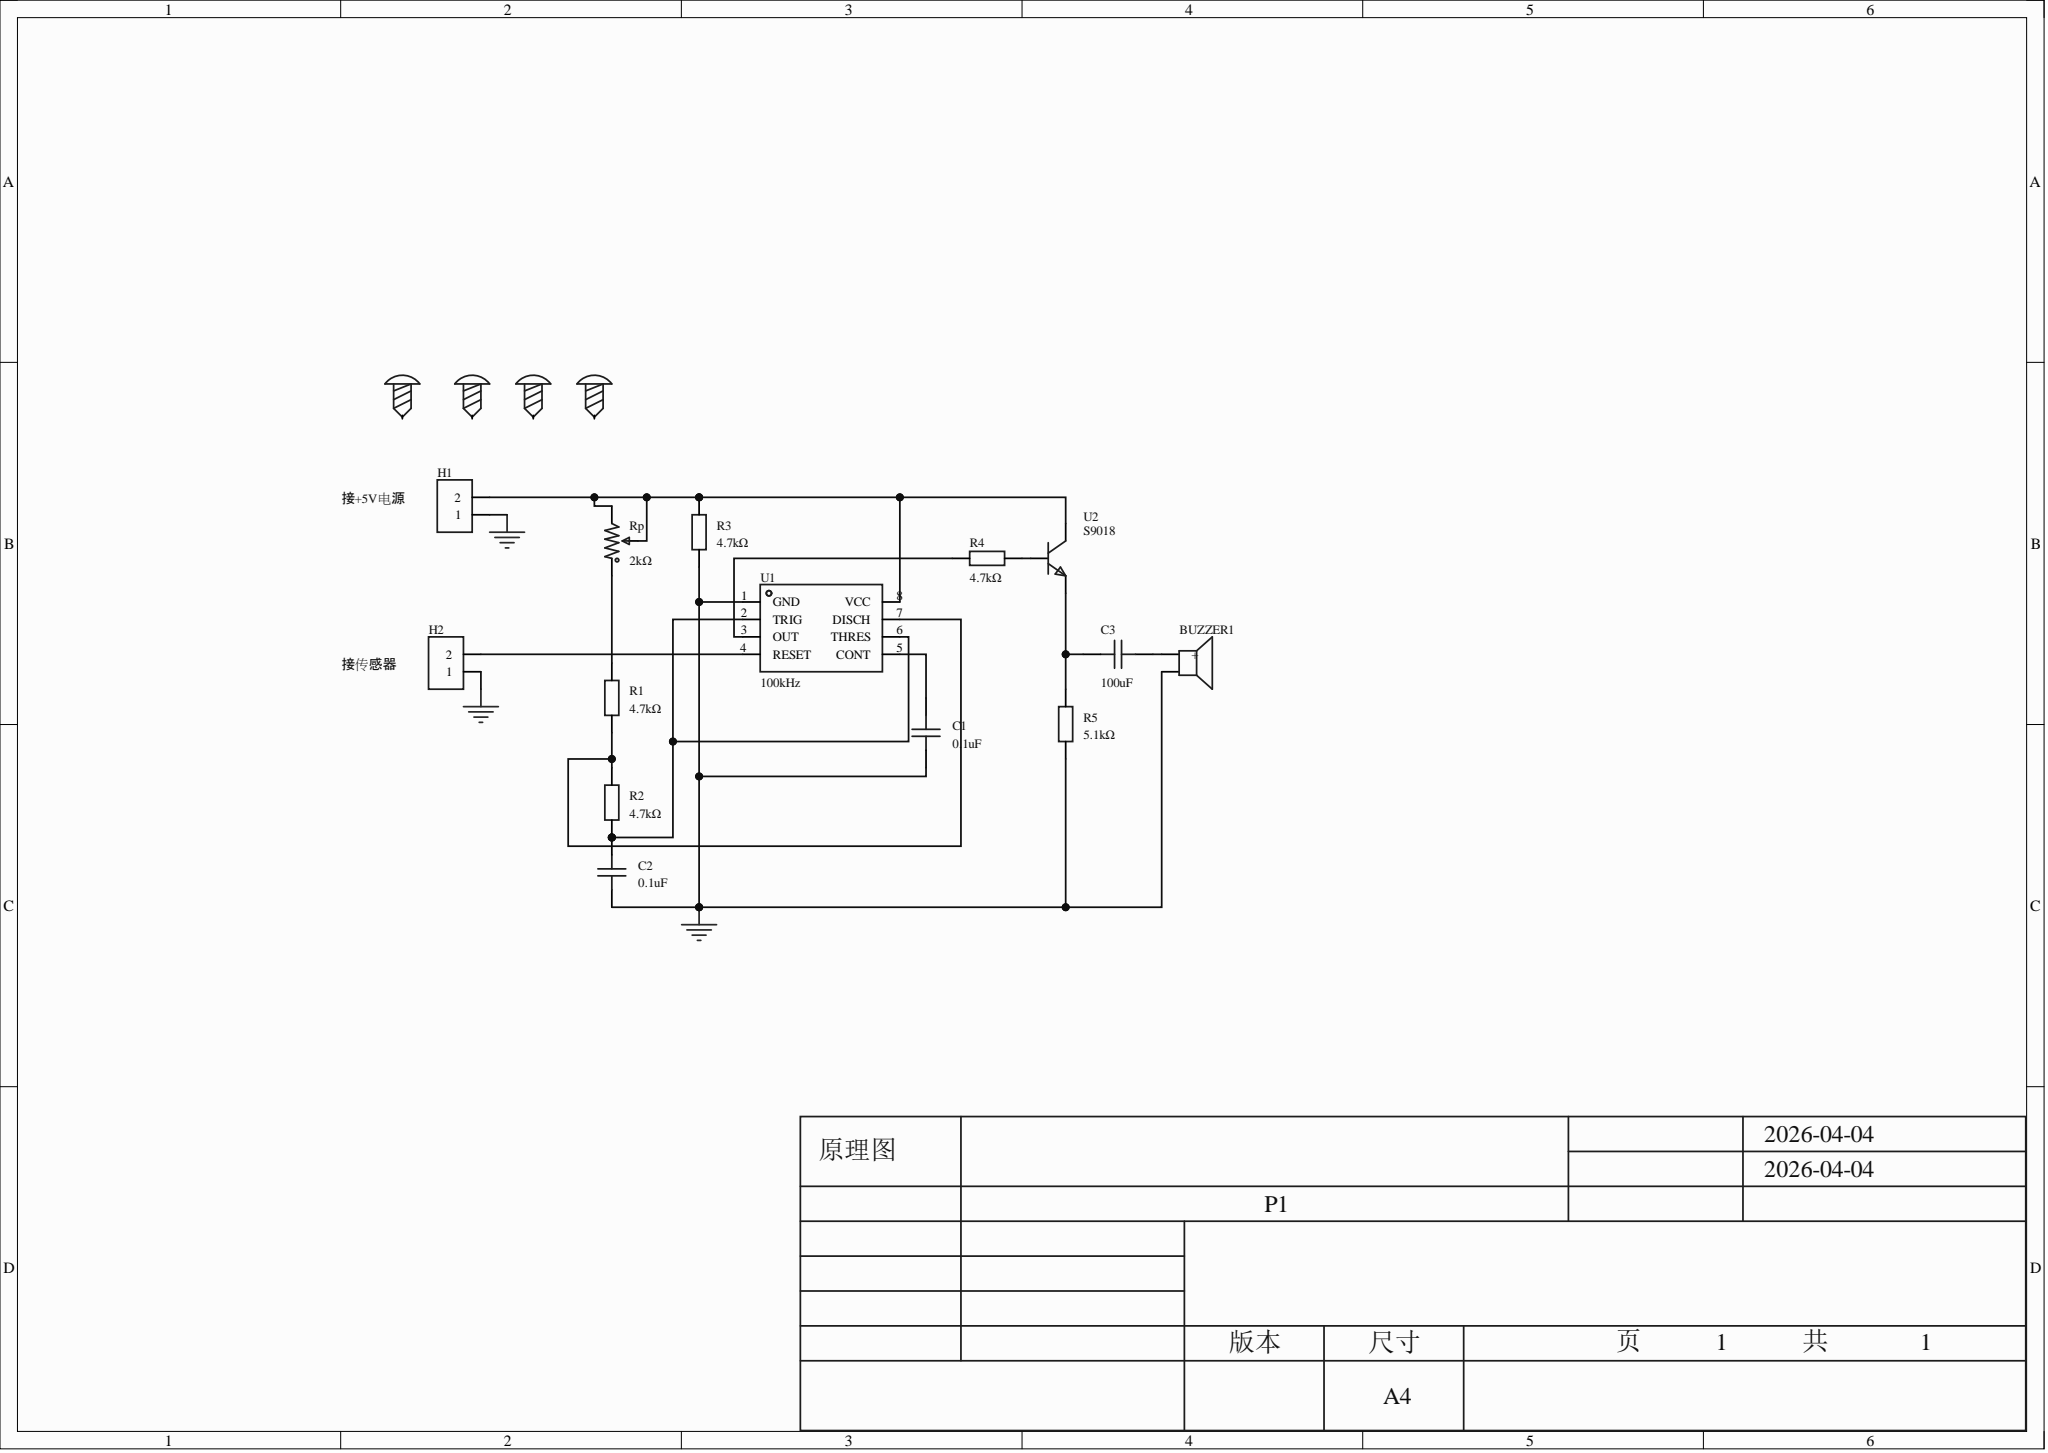Circuit board | Altium Designer | 18 parts | 11 nets
Bill of materials:
Comment,Description,Designator,Footprint,LibRef,Quantity
"","驱动方式:有源(内含驱动线路);构造类型:电磁式;频率:2.7kHz;声压(SPL):85dB;","BUZZER1","BUZ-TH_BD12.0-P7.60-D0.6-FD","TMB12A05_C96093","1"
"0.1uF","容值:100nF;精度:±10%;额定电压:50V;温度系数:X7R;","C1, C2","CAP-TH_L8.5-W5.0-P5.00-D1.2","CT4-0805B104K500F3","2"
"100uF","容值:100nF;精度:±10%;额定电压:50V;温度系数:X7R;","C3","CAP-TH_L8.5-W5.0-P5.00-D1.2","CT4-0805B104K500F3","1"
"","","H1, H2","HDR-TH_2P-P2.54-V-F","HDR-F_2.54_1x2P","2"
"4.7kΩ","","R1, R2, R3, R4","RES-TH_BD2.3-L6.5-P10.50-D0.5","MF1/4W-4.7KΩ±1% T","4"
"5.1kΩ","","R5","RES-TH_BD2.3-L6.5-P10.50-D0.5","MF1/4W-4.7KΩ±1% T","1"
"2kΩ","","Rp","RES-ADJ-TH_3P-L10.0-W10.0-P2.50-BL-BS","3296W-1-102","1"
"","","SCREW1, SCREW2, SCREW3, SCREW4","M2螺丝","M2螺丝","4"
"100kHz","频率:100kHz;","U1","DIP-8_L9.8-W6.6-P2.54-LS7.6-BL","NE555P","1"
"S9018","晶体管类型:NPN;集电极电流(Ic):-;集射极击穿电压(Vceo):25V;功率(Pd):350mW;直流电流增益(hFE@Ic,Vce):60@4mA,10V;","U2","TO-92-3_L4.8-W3.7-P1.27-L","MPSH10_C3197038","1"
Netlist (Protel format):
[
BUZZER1
BUZ-TH_BD12.0-P7.60-D0.6-FD




]
[
C1
CAP-TH_L8.5-W5.0-P5.00-D1.2
0.1uF



]
[
C2
CAP-TH_L8.5-W5.0-P5.00-D1.2
0.1uF



]
[
C3
CAP-TH_L8.5-W5.0-P5.00-D1.2
100uF



]
[
H1
HDR-TH_2P-P2.54-V-F




]
[
H2
HDR-TH_2P-P2.54-V-F




]
[
R1
RES-TH_BD2.3-L6.5-P10.50-D0.5
4.7kΩ



]
[
R2
RES-TH_BD2.3-L6.5-P10.50-D0.5
4.7kΩ



]
[
R3
RES-TH_BD2.3-L6.5-P10.50-D0.5
4.7kΩ



]
[
R4
RES-TH_BD2.3-L6.5-P10.50-D0.5
4.7kΩ



]
[
R5
RES-TH_BD2.3-L6.5-P10.50-D0.5
5.1kΩ



]
[
Rp
RES-ADJ-TH_3P-L10.0-W10.0-P2.50-BL-BS
2kΩ



]
[
SCREW1
M2螺丝




]
[
SCREW2
M2螺丝




]
[
SCREW3
M2螺丝




]
[
SCREW4
M2螺丝




]
[
U1
DIP-8_L9.8-W6.6-P2.54-LS7.6-BL
100kHz



]
[
U2
TO-92-3_L4.8-W3.7-P1.27-L
S9018



]
(
NetR4_2
R4-2
U1-3
)
(
NetR4_1
R4-1
U2-1
)
(
NetR1_2
R1-2
Rp-1
)
(
NetR1_1
R1-1
R2-2
U1-7
)
(
NetH2_2
H2-2
U1-4
)
(
NetH1_2
H1-2
R3-2
Rp-2
Rp-3
U1-8
U2-3
)
(
NetC3_2
C3-2
R5-2
U2-2
)
(
NetC2_2
C2-2
R2-1
U1-2
U1-6
)
(
NetC1_1
C1-1
U1-5
)
(
NetBUZZER1_1
BUZZER1-1
C3-1
)
(
GND
BUZZER1-2
C1-2
C2-1
H1-1
H2-1
R3-1
R5-1
U1-1
)